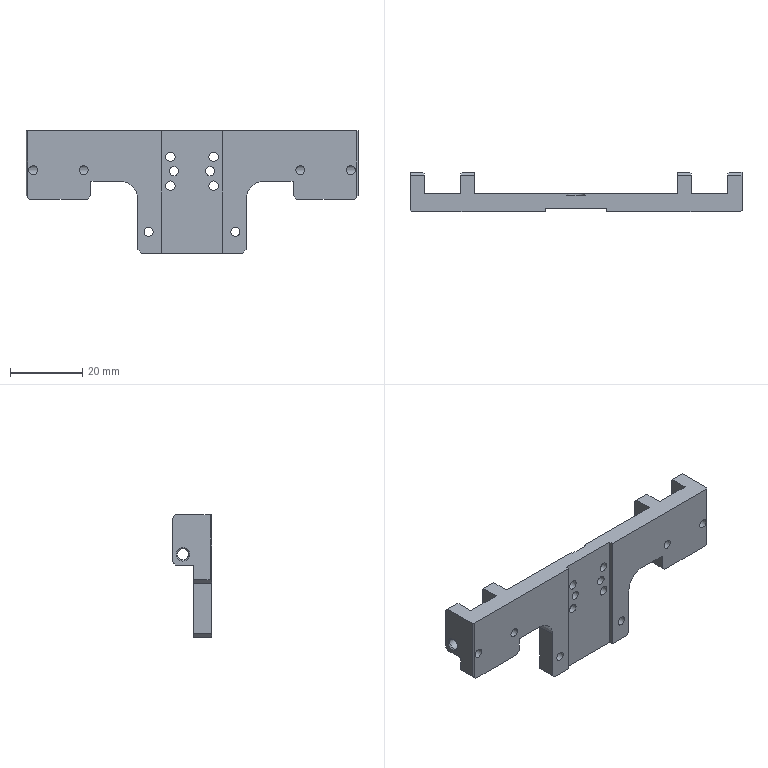Part | 1 solid | 94 faces | box 92 x 11 x 34 mm | volume 10507 mm3 | plane 64 | cylinder 26 | cone 4 | commonest cylinder face diameters 2.5 x8 2.6 x4 3.1 x4 4.3 x4 4 x2 4.2 x2